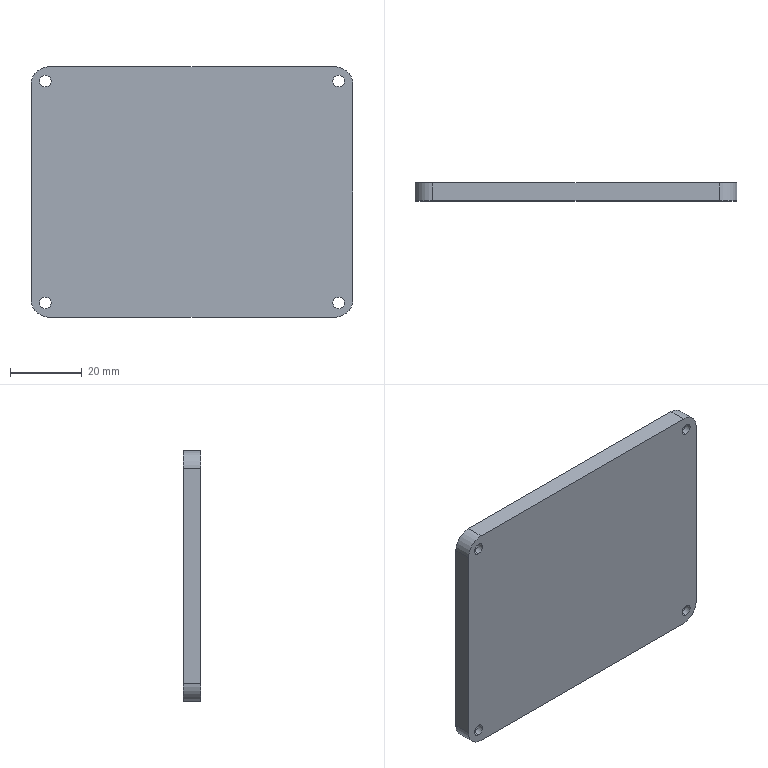Part | SolidWorks | features Extrusion 1, ICE 1 | 1 solid | 30 faces | box 90 x 5 x 70 mm | volume 30997 mm3 | cylinder 20 | plane 10 | commonest cylinder face diameters 3.2 x8 5.8 x8 10 x4
STEP:
#1=CARTESIAN_POINT('',(-41.,1.8,-33.9));
#2=VERTEX_POINT('',#1);
#3=CARTESIAN_POINT('',(-41.,1.8,-28.1));
#4=VERTEX_POINT('',#3);
#5=CARTESIAN_POINT('',(-41.,1.8,-31.));
#6=DIRECTION('',(0.,1.,0.));
#7=DIRECTION('',(0.,0.,1.));
#8=AXIS2_PLACEMENT_3D('',#5,#6,#7);
#9=CIRCLE('',#8,2.9);
#10=EDGE_CURVE('',#2,#4,#9,.T.);
#11=ORIENTED_EDGE('',*,*,#10,.F.);
#12=CARTESIAN_POINT('',(-41.,5.,-33.9));
#13=VERTEX_POINT('',#12);
#14=CARTESIAN_POINT('',(-41.,1.8,-33.9));
#15=DIRECTION('',(0.,1.,0.));
#16=VECTOR('',#15,1000.);
#17=LINE('',#14,#16);
#18=EDGE_CURVE('',#2,#13,#17,.T.);
#19=ORIENTED_EDGE('',*,*,#18,.T.);
#20=CARTESIAN_POINT('',(-41.,5.,-28.1));
#21=VERTEX_POINT('',#20);
#22=CARTESIAN_POINT('',(-41.,5.,-31.));
#23=DIRECTION('',(0.,1.,0.));
#24=DIRECTION('',(0.,0.,1.));
#25=AXIS2_PLACEMENT_3D('',#22,#23,#24);
#26=CIRCLE('',#25,2.9);
#27=EDGE_CURVE('',#13,#21,#26,.T.);
#28=ORIENTED_EDGE('',*,*,#27,.T.);
#29=CARTESIAN_POINT('',(-41.,1.8,-28.1));
#30=DIRECTION('',(0.,1.,0.));
#31=VECTOR('',#30,1000.);
#32=LINE('',#29,#31);
#33=EDGE_CURVE('',#4,#21,#32,.T.);
#34=ORIENTED_EDGE('',*,*,#33,.F.);
#35=EDGE_LOOP('',(#11,#19,#28,#34));
#36=FACE_OUTER_BOUND('',#35,.T.);
#37=CARTESIAN_POINT('',(-41.,1.8,-31.));
#38=DIRECTION('',(0.,1.,0.));
#39=DIRECTION('',(0.,0.,1.));
#40=AXIS2_PLACEMENT_3D('',#37,#38,#39);
#41=CYLINDRICAL_SURFACE('',#40,2.9);
#42=ADVANCED_FACE('',(#36),#41,.F.);
#43=CARTESIAN_POINT('',(-41.,1.8,28.1));
#44=VERTEX_POINT('',#43);
#45=CARTESIAN_POINT('',(-41.,1.8,33.9));
#46=VERTEX_POINT('',#45);
#47=CARTESIAN_POINT('',(-41.,1.8,31.));
#48=DIRECTION('',(0.,1.,0.));
#49=DIRECTION('',(0.,0.,1.));
#50=AXIS2_PLACEMENT_3D('',#47,#48,#49);
#51=CIRCLE('',#50,2.9);
#52=EDGE_CURVE('',#44,#46,#51,.T.);
#53=ORIENTED_EDGE('',*,*,#52,.F.);
#54=CARTESIAN_POINT('',(-41.,5.,28.1));
#55=VERTEX_POINT('',#54);
#56=CARTESIAN_POINT('',(-41.,1.8,28.1));
#57=DIRECTION('',(0.,1.,0.));
#58=VECTOR('',#57,1000.);
#59=LINE('',#56,#58);
#60=EDGE_CURVE('',#44,#55,#59,.T.);
#61=ORIENTED_EDGE('',*,*,#60,.T.);
#62=CARTESIAN_POINT('',(-41.,5.,33.9));
#63=VERTEX_POINT('',#62);
#64=CARTESIAN_POINT('',(-41.,5.,31.));
#65=DIRECTION('',(0.,1.,0.));
#66=DIRECTION('',(0.,0.,1.));
#67=AXIS2_PLACEMENT_3D('',#64,#65,#66);
#68=CIRCLE('',#67,2.9);
#69=EDGE_CURVE('',#55,#63,#68,.T.);
#70=ORIENTED_EDGE('',*,*,#69,.T.);
#71=CARTESIAN_POINT('',(-41.,1.8,33.9));
#72=DIRECTION('',(0.,1.,0.));
#73=VECTOR('',#72,1000.);
#74=LINE('',#71,#73);
#75=EDGE_CURVE('',#46,#63,#74,.T.);
#76=ORIENTED_EDGE('',*,*,#75,.F.);
#77=EDGE_LOOP('',(#53,#61,#70,#76));
#78=FACE_OUTER_BOUND('',#77,.T.);
#79=CARTESIAN_POINT('',(-41.,1.8,31.));
#80=DIRECTION('',(0.,1.,0.));
#81=DIRECTION('',(0.,0.,1.));
#82=AXIS2_PLACEMENT_3D('',#79,#80,#81);
#83=CYLINDRICAL_SURFACE('',#82,2.9);
#84=ADVANCED_FACE('',(#78),#83,.F.);
#85=CARTESIAN_POINT('',(41.,1.8,28.1));
#86=VERTEX_POINT('',#85);
#87=CARTESIAN_POINT('',(41.,1.8,33.9));
#88=VERTEX_POINT('',#87);
#89=CARTESIAN_POINT('',(41.,1.8,31.));
#90=DIRECTION('',(0.,1.,0.));
#91=DIRECTION('',(0.,0.,1.));
#92=AXIS2_PLACEMENT_3D('',#89,#90,#91);
#93=CIRCLE('',#92,2.9);
#94=EDGE_CURVE('',#86,#88,#93,.T.);
#95=ORIENTED_EDGE('',*,*,#94,.F.);
#96=CARTESIAN_POINT('',(41.,5.,28.1));
#97=VERTEX_POINT('',#96);
#98=CARTESIAN_POINT('',(41.,1.8,28.1));
#99=DIRECTION('',(0.,1.,0.));
#100=VECTOR('',#99,1000.);
#101=LINE('',#98,#100);
#102=EDGE_CURVE('',#86,#97,#101,.T.);
#103=ORIENTED_EDGE('',*,*,#102,.T.);
#104=CARTESIAN_POINT('',(41.,5.,33.9));
#105=VERTEX_POINT('',#104);
#106=CARTESIAN_POINT('',(41.,5.,31.));
#107=DIRECTION('',(0.,1.,0.));
#108=DIRECTION('',(0.,0.,1.));
#109=AXIS2_PLACEMENT_3D('',#106,#107,#108);
#110=CIRCLE('',#109,2.9);
#111=EDGE_CURVE('',#97,#105,#110,.T.);
#112=ORIENTED_EDGE('',*,*,#111,.T.);
#113=CARTESIAN_POINT('',(41.,1.8,33.9));
#114=DIRECTION('',(0.,1.,0.));
#115=VECTOR('',#114,1000.);
#116=LINE('',#113,#115);
#117=EDGE_CURVE('',#88,#105,#116,.T.);
#118=ORIENTED_EDGE('',*,*,#117,.F.);
#119=EDGE_LOOP('',(#95,#103,#112,#118));
#120=FACE_OUTER_BOUND('',#119,.T.);
#121=CARTESIAN_POINT('',(41.,1.8,31.));
#122=DIRECTION('',(0.,1.,0.));
#123=DIRECTION('',(0.,0.,1.));
#124=AXIS2_PLACEMENT_3D('',#121,#122,#123);
#125=CYLINDRICAL_SURFACE('',#124,2.9);
#126=ADVANCED_FACE('',(#120),#125,.F.);
#127=CARTESIAN_POINT('',(41.,1.8,-33.9));
#128=VERTEX_POINT('',#127);
#129=CARTESIAN_POINT('',(41.,1.8,-28.1));
#130=VERTEX_POINT('',#129);
#131=CARTESIAN_POINT('',(41.,1.8,-31.));
#132=DIRECTION('',(0.,1.,0.));
#133=DIRECTION('',(0.,0.,1.));
#134=AXIS2_PLACEMENT_3D('',#131,#132,#133);
#135=CIRCLE('',#134,2.9);
#136=EDGE_CURVE('',#128,#130,#135,.T.);
#137=ORIENTED_EDGE('',*,*,#136,.F.);
#138=CARTESIAN_POINT('',(41.,5.,-33.9));
#139=VERTEX_POINT('',#138);
#140=CARTESIAN_POINT('',(41.,1.8,-33.9));
#141=DIRECTION('',(0.,1.,0.));
#142=VECTOR('',#141,1000.);
#143=LINE('',#140,#142);
#144=EDGE_CURVE('',#128,#139,#143,.T.);
#145=ORIENTED_EDGE('',*,*,#144,.T.);
#146=CARTESIAN_POINT('',(41.,5.,-28.1));
#147=VERTEX_POINT('',#146);
#148=CARTESIAN_POINT('',(41.,5.,-31.));
#149=DIRECTION('',(0.,1.,0.));
#150=DIRECTION('',(0.,0.,1.));
#151=AXIS2_PLACEMENT_3D('',#148,#149,#150);
#152=CIRCLE('',#151,2.9);
#153=EDGE_CURVE('',#139,#147,#152,.T.);
#154=ORIENTED_EDGE('',*,*,#153,.T.);
#155=CARTESIAN_POINT('',(41.,1.8,-28.1));
#156=DIRECTION('',(0.,1.,0.));
#157=VECTOR('',#156,1000.);
#158=LINE('',#155,#157);
#159=EDGE_CURVE('',#130,#147,#158,.T.);
#160=ORIENTED_EDGE('',*,*,#159,.F.);
#161=EDGE_LOOP('',(#137,#145,#154,#160));
#162=FACE_OUTER_BOUND('',#161,.T.);
#163=CARTESIAN_POINT('',(41.,1.8,-31.));
#164=DIRECTION('',(0.,1.,0.));
#165=DIRECTION('',(0.,0.,1.));
#166=AXIS2_PLACEMENT_3D('',#163,#164,#165);
#167=CYLINDRICAL_SURFACE('',#166,2.9);
#168=ADVANCED_FACE('',(#162),#167,.F.);
#169=CARTESIAN_POINT('',(41.,1.8,-32.6));
#170=VERTEX_POINT('',#169);
#171=CARTESIAN_POINT('',(41.,1.8,-29.4));
#172=VERTEX_POINT('',#171);
#173=CARTESIAN_POINT('',(41.,1.8,-31.));
#174=DIRECTION('',(0.,1.,0.));
#175=DIRECTION('',(0.,0.,1.));
#176=AXIS2_PLACEMENT_3D('',#173,#174,#175);
#177=CIRCLE('',#176,1.6);
#178=EDGE_CURVE('',#170,#172,#177,.T.);
#179=ORIENTED_EDGE('',*,*,#178,.T.);
#180=CARTESIAN_POINT('',(41.,0.,-29.4));
#181=VERTEX_POINT('',#180);
#182=CARTESIAN_POINT('',(41.,5.,-29.4));
#183=DIRECTION('',(0.,-1.,0.));
#184=VECTOR('',#183,1000.);
#185=LINE('',#182,#184);
#186=EDGE_CURVE('',#172,#181,#185,.T.);
#187=ORIENTED_EDGE('',*,*,#186,.T.);
#188=CARTESIAN_POINT('',(41.,0.,-32.6));
#189=VERTEX_POINT('',#188);
#190=CARTESIAN_POINT('',(41.,0.,-31.));
#191=DIRECTION('',(0.,1.,0.));
#192=DIRECTION('',(0.,0.,1.));
#193=AXIS2_PLACEMENT_3D('',#190,#191,#192);
#194=CIRCLE('',#193,1.6);
#195=EDGE_CURVE('',#189,#181,#194,.T.);
#196=ORIENTED_EDGE('',*,*,#195,.F.);
#197=CARTESIAN_POINT('',(41.,5.,-32.6));
#198=DIRECTION('',(0.,-1.,0.));
#199=VECTOR('',#198,1000.);
#200=LINE('',#197,#199);
#201=EDGE_CURVE('',#170,#189,#200,.T.);
#202=ORIENTED_EDGE('',*,*,#201,.F.);
#203=EDGE_LOOP('',(#179,#187,#196,#202));
#204=FACE_OUTER_BOUND('',#203,.T.);
#205=CARTESIAN_POINT('',(41.,5.,-31.));
#206=DIRECTION('',(0.,-1.,0.));
#207=DIRECTION('',(0.,0.,-1.));
#208=AXIS2_PLACEMENT_3D('',#205,#206,#207);
#209=CYLINDRICAL_SURFACE('',#208,1.6);
#210=ADVANCED_FACE('',(#204),#209,.F.);
#211=CARTESIAN_POINT('',(41.,1.8,29.4));
#212=VERTEX_POINT('',#211);
#213=CARTESIAN_POINT('',(41.,1.8,32.6));
#214=VERTEX_POINT('',#213);
#215=CARTESIAN_POINT('',(41.,1.8,31.));
#216=DIRECTION('',(0.,1.,0.));
#217=DIRECTION('',(0.,0.,1.));
#218=AXIS2_PLACEMENT_3D('',#215,#216,#217);
#219=CIRCLE('',#218,1.6);
#220=EDGE_CURVE('',#212,#214,#219,.T.);
#221=ORIENTED_EDGE('',*,*,#220,.T.);
#222=CARTESIAN_POINT('',(41.,0.,32.6));
#223=VERTEX_POINT('',#222);
#224=CARTESIAN_POINT('',(41.,5.,32.6));
#225=DIRECTION('',(0.,-1.,0.));
#226=VECTOR('',#225,1000.);
#227=LINE('',#224,#226);
#228=EDGE_CURVE('',#214,#223,#227,.T.);
#229=ORIENTED_EDGE('',*,*,#228,.T.);
#230=CARTESIAN_POINT('',(41.,0.,29.4));
#231=VERTEX_POINT('',#230);
#232=CARTESIAN_POINT('',(41.,0.,31.));
#233=DIRECTION('',(0.,1.,0.));
#234=DIRECTION('',(0.,0.,1.));
#235=AXIS2_PLACEMENT_3D('',#232,#233,#234);
#236=CIRCLE('',#235,1.6);
#237=EDGE_CURVE('',#231,#223,#236,.T.);
#238=ORIENTED_EDGE('',*,*,#237,.F.);
#239=CARTESIAN_POINT('',(41.,5.,29.4));
#240=DIRECTION('',(0.,-1.,0.));
#241=VECTOR('',#240,1000.);
#242=LINE('',#239,#241);
#243=EDGE_CURVE('',#212,#231,#242,.T.);
#244=ORIENTED_EDGE('',*,*,#243,.F.);
#245=EDGE_LOOP('',(#221,#229,#238,#244));
#246=FACE_OUTER_BOUND('',#245,.T.);
#247=CARTESIAN_POINT('',(41.,5.,31.));
#248=DIRECTION('',(0.,-1.,0.));
#249=DIRECTION('',(0.,0.,-1.));
#250=AXIS2_PLACEMENT_3D('',#247,#248,#249);
#251=CYLINDRICAL_SURFACE('',#250,1.6);
#252=ADVANCED_FACE('',(#246),#251,.F.);
#253=CARTESIAN_POINT('',(-41.,1.8,29.4));
#254=VERTEX_POINT('',#253);
#255=CARTESIAN_POINT('',(-41.,1.8,32.6));
#256=VERTEX_POINT('',#255);
#257=CARTESIAN_POINT('',(-41.,1.8,31.));
#258=DIRECTION('',(0.,1.,0.));
#259=DIRECTION('',(0.,0.,1.));
#260=AXIS2_PLACEMENT_3D('',#257,#258,#259);
#261=CIRCLE('',#260,1.6);
#262=EDGE_CURVE('',#254,#256,#261,.T.);
#263=ORIENTED_EDGE('',*,*,#262,.T.);
#264=CARTESIAN_POINT('',(-41.,0.,32.6));
#265=VERTEX_POINT('',#264);
#266=CARTESIAN_POINT('',(-41.,5.,32.6));
#267=DIRECTION('',(0.,-1.,0.));
#268=VECTOR('',#267,1000.);
#269=LINE('',#266,#268);
#270=EDGE_CURVE('',#256,#265,#269,.T.);
#271=ORIENTED_EDGE('',*,*,#270,.T.);
#272=CARTESIAN_POINT('',(-41.,0.,29.4));
#273=VERTEX_POINT('',#272);
#274=CARTESIAN_POINT('',(-41.,0.,31.));
#275=DIRECTION('',(0.,1.,0.));
#276=DIRECTION('',(0.,0.,1.));
#277=AXIS2_PLACEMENT_3D('',#274,#275,#276);
#278=CIRCLE('',#277,1.6);
#279=EDGE_CURVE('',#273,#265,#278,.T.);
#280=ORIENTED_EDGE('',*,*,#279,.F.);
#281=CARTESIAN_POINT('',(-41.,5.,29.4));
#282=DIRECTION('',(0.,-1.,0.));
#283=VECTOR('',#282,1000.);
#284=LINE('',#281,#283);
#285=EDGE_CURVE('',#254,#273,#284,.T.);
#286=ORIENTED_EDGE('',*,*,#285,.F.);
#287=EDGE_LOOP('',(#263,#271,#280,#286));
#288=FACE_OUTER_BOUND('',#287,.T.);
#289=CARTESIAN_POINT('',(-41.,5.,31.));
#290=DIRECTION('',(0.,-1.,0.));
#291=DIRECTION('',(0.,0.,-1.));
#292=AXIS2_PLACEMENT_3D('',#289,#290,#291);
#293=CYLINDRICAL_SURFACE('',#292,1.6);
#294=ADVANCED_FACE('',(#288),#293,.F.);
#295=CARTESIAN_POINT('',(-41.,1.8,-32.6));
#296=VERTEX_POINT('',#295);
#297=CARTESIAN_POINT('',(-41.,1.8,-29.4));
#298=VERTEX_POINT('',#297);
#299=CARTESIAN_POINT('',(-41.,1.8,-31.));
#300=DIRECTION('',(0.,1.,0.));
#301=DIRECTION('',(0.,0.,1.));
#302=AXIS2_PLACEMENT_3D('',#299,#300,#301);
#303=CIRCLE('',#302,1.6);
#304=EDGE_CURVE('',#296,#298,#303,.T.);
#305=ORIENTED_EDGE('',*,*,#304,.T.);
#306=CARTESIAN_POINT('',(-41.,0.,-29.4));
#307=VERTEX_POINT('',#306);
#308=CARTESIAN_POINT('',(-41.,5.,-29.4));
#309=DIRECTION('',(0.,-1.,0.));
#310=VECTOR('',#309,1000.);
#311=LINE('',#308,#310);
#312=EDGE_CURVE('',#298,#307,#311,.T.);
#313=ORIENTED_EDGE('',*,*,#312,.T.);
#314=CARTESIAN_POINT('',(-41.,0.,-32.6));
#315=VERTEX_POINT('',#314);
#316=CARTESIAN_POINT('',(-41.,0.,-31.));
#317=DIRECTION('',(0.,1.,0.));
#318=DIRECTION('',(0.,0.,1.));
#319=AXIS2_PLACEMENT_3D('',#316,#317,#318);
#320=CIRCLE('',#319,1.6);
#321=EDGE_CURVE('',#315,#307,#320,.T.);
#322=ORIENTED_EDGE('',*,*,#321,.F.);
#323=CARTESIAN_POINT('',(-41.,5.,-32.6));
#324=DIRECTION('',(0.,-1.,0.));
#325=VECTOR('',#324,1000.);
#326=LINE('',#323,#325);
#327=EDGE_CURVE('',#296,#315,#326,.T.);
#328=ORIENTED_EDGE('',*,*,#327,.F.);
#329=EDGE_LOOP('',(#305,#313,#322,#328));
#330=FACE_OUTER_BOUND('',#329,.T.);
#331=CARTESIAN_POINT('',(-41.,5.,-31.));
#332=DIRECTION('',(0.,-1.,0.));
#333=DIRECTION('',(0.,0.,-1.));
#334=AXIS2_PLACEMENT_3D('',#331,#332,#333);
#335=CYLINDRICAL_SURFACE('',#334,1.6);
#336=ADVANCED_FACE('',(#330),#335,.F.);
#337=ORIENTED_EDGE('',*,*,#312,.F.);
#338=CARTESIAN_POINT('',(-41.,1.8,-31.));
#339=DIRECTION('',(0.,1.,0.));
#340=DIRECTION('',(0.,0.,1.));
#341=AXIS2_PLACEMENT_3D('',#338,#339,#340);
#342=CIRCLE('',#341,1.6);
#343=EDGE_CURVE('',#298,#296,#342,.T.);
#344=ORIENTED_EDGE('',*,*,#343,.T.);
#345=ORIENTED_EDGE('',*,*,#327,.T.);
#346=CARTESIAN_POINT('',(-41.,0.,-31.));
#347=DIRECTION('',(0.,1.,0.));
#348=DIRECTION('',(0.,0.,1.));
#349=AXIS2_PLACEMENT_3D('',#346,#347,#348);
#350=CIRCLE('',#349,1.6);
#351=EDGE_CURVE('',#307,#315,#350,.T.);
#352=ORIENTED_EDGE('',*,*,#351,.F.);
#353=EDGE_LOOP('',(#337,#344,#345,#352));
#354=FACE_OUTER_BOUND('',#353,.T.);
#355=CARTESIAN_POINT('',(-41.,5.,-31.));
#356=DIRECTION('',(0.,-1.,0.));
#357=DIRECTION('',(0.,0.,-1.));
#358=AXIS2_PLACEMENT_3D('',#355,#356,#357);
#359=CYLINDRICAL_SURFACE('',#358,1.6);
#360=ADVANCED_FACE('',(#354),#359,.F.);
#361=ORIENTED_EDGE('',*,*,#270,.F.);
#362=CARTESIAN_POINT('',(-41.,1.8,31.));
#363=DIRECTION('',(0.,1.,0.));
#364=DIRECTION('',(0.,0.,1.));
#365=AXIS2_PLACEMENT_3D('',#362,#363,#364);
#366=CIRCLE('',#365,1.6);
#367=EDGE_CURVE('',#256,#254,#366,.T.);
#368=ORIENTED_EDGE('',*,*,#367,.T.);
#369=ORIENTED_EDGE('',*,*,#285,.T.);
#370=CARTESIAN_POINT('',(-41.,0.,31.));
#371=DIRECTION('',(0.,1.,0.));
#372=DIRECTION('',(0.,0.,1.));
#373=AXIS2_PLACEMENT_3D('',#370,#371,#372);
#374=CIRCLE('',#373,1.6);
#375=EDGE_CURVE('',#265,#273,#374,.T.);
#376=ORIENTED_EDGE('',*,*,#375,.F.);
#377=EDGE_LOOP('',(#361,#368,#369,#376));
#378=FACE_OUTER_BOUND('',#377,.T.);
#379=CARTESIAN_POINT('',(-41.,5.,31.));
#380=DIRECTION('',(0.,-1.,0.));
#381=DIRECTION('',(0.,0.,-1.));
#382=AXIS2_PLACEMENT_3D('',#379,#380,#381);
#383=CYLINDRICAL_SURFACE('',#382,1.6);
#384=ADVANCED_FACE('',(#378),#383,.F.);
#385=ORIENTED_EDGE('',*,*,#228,.F.);
#386=CARTESIAN_POINT('',(41.,1.8,31.));
#387=DIRECTION('',(0.,1.,0.));
#388=DIRECTION('',(0.,0.,1.));
#389=AXIS2_PLACEMENT_3D('',#386,#387,#388);
#390=CIRCLE('',#389,1.6);
#391=EDGE_CURVE('',#214,#212,#390,.T.);
#392=ORIENTED_EDGE('',*,*,#391,.T.);
#393=ORIENTED_EDGE('',*,*,#243,.T.);
#394=CARTESIAN_POINT('',(41.,0.,31.));
#395=DIRECTION('',(0.,1.,0.));
#396=DIRECTION('',(0.,0.,1.));
#397=AXIS2_PLACEMENT_3D('',#394,#395,#396);
#398=CIRCLE('',#397,1.6);
#399=EDGE_CURVE('',#223,#231,#398,.T.);
#400=ORIENTED_EDGE('',*,*,#399,.F.);
#401=EDGE_LOOP('',(#385,#392,#393,#400));
#402=FACE_OUTER_BOUND('',#401,.T.);
#403=CARTESIAN_POINT('',(41.,5.,31.));
#404=DIRECTION('',(0.,-1.,0.));
#405=DIRECTION('',(0.,0.,-1.));
#406=AXIS2_PLACEMENT_3D('',#403,#404,#405);
#407=CYLINDRICAL_SURFACE('',#406,1.6);
#408=ADVANCED_FACE('',(#402),#407,.F.);
#409=ORIENTED_EDGE('',*,*,#186,.F.);
#410=CARTESIAN_POINT('',(41.,1.8,-31.));
#411=DIRECTION('',(0.,1.,0.));
#412=DIRECTION('',(0.,0.,1.));
#413=AXIS2_PLACEMENT_3D('',#410,#411,#412);
#414=CIRCLE('',#413,1.6);
#415=EDGE_CURVE('',#172,#170,#414,.T.);
#416=ORIENTED_EDGE('',*,*,#415,.T.);
#417=ORIENTED_EDGE('',*,*,#201,.T.);
#418=CARTESIAN_POINT('',(41.,0.,-31.));
#419=DIRECTION('',(0.,1.,0.));
#420=DIRECTION('',(0.,0.,1.));
#421=AXIS2_PLACEMENT_3D('',#418,#419,#420);
#422=CIRCLE('',#421,1.6);
#423=EDGE_CURVE('',#181,#189,#422,.T.);
#424=ORIENTED_EDGE('',*,*,#423,.F.);
#425=EDGE_LOOP('',(#409,#416,#417,#424));
#426=FACE_OUTER_BOUND('',#425,.T.);
#427=CARTESIAN_POINT('',(41.,5.,-31.));
#428=DIRECTION('',(0.,-1.,0.));
#429=DIRECTION('',(0.,0.,-1.));
#430=AXIS2_PLACEMENT_3D('',#427,#428,#429);
#431=CYLINDRICAL_SURFACE('',#430,1.6);
#432=ADVANCED_FACE('',(#426),#431,.F.);
#433=CARTESIAN_POINT('',(41.,5.,31.));
#434=DIRECTION('',(0.,1.,0.));
#435=DIRECTION('',(0.,0.,1.));
#436=AXIS2_PLACEMENT_3D('',#433,#434,#435);
#437=CIRCLE('',#436,2.9);
#438=EDGE_CURVE('',#105,#97,#437,.T.);
#439=ORIENTED_EDGE('',*,*,#438,.F.);
#440=ORIENTED_EDGE('',*,*,#111,.F.);
#441=EDGE_LOOP('',(#439,#440));
#442=FACE_BOUND('',#441,.T.);
#443=CARTESIAN_POINT('',(-41.,5.,31.));
#444=DIRECTION('',(0.,1.,0.));
#445=DIRECTION('',(0.,0.,1.));
#446=AXIS2_PLACEMENT_3D('',#443,#444,#445);
#447=CIRCLE('',#446,2.9);
#448=EDGE_CURVE('',#63,#55,#447,.T.);
#449=ORIENTED_EDGE('',*,*,#448,.F.);
#450=ORIENTED_EDGE('',*,*,#69,.F.);
#451=EDGE_LOOP('',(#449,#450));
#452=FACE_BOUND('',#451,.T.);
#453=CARTESIAN_POINT('',(-41.,5.,-31.));
#454=DIRECTION('',(0.,1.,0.));
#455=DIRECTION('',(0.,0.,1.));
#456=AXIS2_PLACEMENT_3D('',#453,#454,#455);
#457=CIRCLE('',#456,2.9);
#458=EDGE_CURVE('',#21,#13,#457,.T.);
#459=ORIENTED_EDGE('',*,*,#458,.F.);
#460=ORIENTED_EDGE('',*,*,#27,.F.);
#461=EDGE_LOOP('',(#459,#460));
#462=FACE_BOUND('',#461,.T.);
#463=CARTESIAN_POINT('',(41.,5.,-31.));
#464=DIRECTION('',(0.,1.,0.));
#465=DIRECTION('',(0.,0.,1.));
#466=AXIS2_PLACEMENT_3D('',#463,#464,#465);
#467=CIRCLE('',#466,2.9);
#468=EDGE_CURVE('',#147,#139,#467,.T.);
#469=ORIENTED_EDGE('',*,*,#468,.F.);
#470=ORIENTED_EDGE('',*,*,#153,.F.);
#471=EDGE_LOOP('',(#469,#470));
#472=FACE_BOUND('',#471,.T.);
#473=CARTESIAN_POINT('',(-45.,5.,30.));
#474=VERTEX_POINT('',#473);
#475=CARTESIAN_POINT('',(-40.,5.,35.));
#476=VERTEX_POINT('',#475);
#477=CARTESIAN_POINT('',(-40.,5.,30.));
#478=DIRECTION('',(0.,1.,0.));
#479=DIRECTION('',(0.,0.,-1.));
#480=AXIS2_PLACEMENT_3D('',#477,#478,#479);
#481=CIRCLE('',#480,5.);
#482=EDGE_CURVE('',#474,#476,#481,.T.);
#483=ORIENTED_EDGE('',*,*,#482,.T.);
#484=CARTESIAN_POINT('',(40.,5.,35.));
#485=VERTEX_POINT('',#484);
#486=CARTESIAN_POINT('',(-40.,5.,35.));
#487=DIRECTION('',(1.,0.,0.));
#488=VECTOR('',#487,1000.);
#489=LINE('',#486,#488);
#490=EDGE_CURVE('',#476,#485,#489,.T.);
#491=ORIENTED_EDGE('',*,*,#490,.T.);
#492=CARTESIAN_POINT('',(45.,5.,30.));
#493=VERTEX_POINT('',#492);
#494=CARTESIAN_POINT('',(40.,5.,30.));
#495=DIRECTION('',(0.,1.,0.));
#496=DIRECTION('',(0.,0.,1.));
#497=AXIS2_PLACEMENT_3D('',#494,#495,#496);
#498=CIRCLE('',#497,5.);
#499=EDGE_CURVE('',#485,#493,#498,.T.);
#500=ORIENTED_EDGE('',*,*,#499,.T.);
#501=CARTESIAN_POINT('',(45.,5.,-30.));
#502=VERTEX_POINT('',#501);
#503=CARTESIAN_POINT('',(45.,5.,30.));
#504=DIRECTION('',(0.,0.,-1.));
#505=VECTOR('',#504,1000.);
#506=LINE('',#503,#505);
#507=EDGE_CURVE('',#493,#502,#506,.T.);
#508=ORIENTED_EDGE('',*,*,#507,.T.);
#509=CARTESIAN_POINT('',(40.,5.,-35.));
#510=VERTEX_POINT('',#509);
#511=CARTESIAN_POINT('',(40.,5.,-30.));
#512=DIRECTION('',(0.,1.,0.));
#513=DIRECTION('',(0.,0.,-1.));
#514=AXIS2_PLACEMENT_3D('',#511,#512,#513);
#515=CIRCLE('',#514,5.);
#516=EDGE_CURVE('',#502,#510,#515,.T.);
#517=ORIENTED_EDGE('',*,*,#516,.T.);
#518=CARTESIAN_POINT('',(-40.,5.,-35.));
#519=VERTEX_POINT('',#518);
#520=CARTESIAN_POINT('',(-40.,5.,-35.));
#521=DIRECTION('',(-1.,0.,0.));
#522=VECTOR('',#521,1000.);
#523=LINE('',#520,#522);
#524=EDGE_CURVE('',#510,#519,#523,.T.);
#525=ORIENTED_EDGE('',*,*,#524,.T.);
#526=CARTESIAN_POINT('',(-45.,5.,-30.));
#527=VERTEX_POINT('',#526);
#528=CARTESIAN_POINT('',(-40.,5.,-30.));
#529=DIRECTION('',(0.,1.,0.));
#530=DIRECTION('',(0.,0.,-1.));
#531=AXIS2_PLACEMENT_3D('',#528,#529,#530);
#532=CIRCLE('',#531,5.);
#533=EDGE_CURVE('',#519,#527,#532,.T.);
#534=ORIENTED_EDGE('',*,*,#533,.T.);
#535=CARTESIAN_POINT('',(-45.,5.,30.));
#536=DIRECTION('',(0.,0.,1.));
#537=VECTOR('',#536,1000.);
#538=LINE('',#535,#537);
#539=EDGE_CURVE('',#527,#474,#538,.T.);
#540=ORIENTED_EDGE('',*,*,#539,.T.);
#541=EDGE_LOOP('',(#483,#491,#500,#508,#517,#525,#534,#540));
#542=FACE_OUTER_BOUND('',#541,.T.);
#543=CARTESIAN_POINT('',(-40.,5.,30.));
#544=DIRECTION('',(0.,-1.,0.));
#545=DIRECTION('',(0.,0.,-1.));
#546=AXIS2_PLACEMENT_3D('',#543,#544,#545);
#547=PLANE('',#546);
#548=ADVANCED_FACE('',(#442,#452,#462,#472,#542),#547,.F.);
#549=ORIENTED_EDGE('',*,*,#237,.T.);
#550=ORIENTED_EDGE('',*,*,#399,.T.);
#551=EDGE_LOOP('',(#549,#550));
#552=FACE_BOUND('',#551,.T.);
#553=ORIENTED_EDGE('',*,*,#321,.T.);
#554=ORIENTED_EDGE('',*,*,#351,.T.);
#555=EDGE_LOOP('',(#553,#554));
#556=FACE_BOUND('',#555,.T.);
#557=CARTESIAN_POINT('',(-45.,0.,30.));
#558=VERTEX_POINT('',#557);
#559=CARTESIAN_POINT('',(-40.,0.,35.));
#560=VERTEX_POINT('',#559);
#561=CARTESIAN_POINT('',(-40.,0.,30.));
#562=DIRECTION('',(0.,1.,0.));
#563=DIRECTION('',(0.,0.,-1.));
#564=AXIS2_PLACEMENT_3D('',#561,#562,#563);
#565=CIRCLE('',#564,5.);
#566=EDGE_CURVE('',#558,#560,#565,.T.);
#567=ORIENTED_EDGE('',*,*,#566,.F.);
#568=CARTESIAN_POINT('',(-45.,0.,-30.));
#569=VERTEX_POINT('',#568);
#570=CARTESIAN_POINT('',(-45.,0.,30.));
#571=DIRECTION('',(0.,0.,1.));
#572=VECTOR('',#571,1000.);
#573=LINE('',#570,#572);
#574=EDGE_CURVE('',#569,#558,#573,.T.);
#575=ORIENTED_EDGE('',*,*,#574,.F.);
#576=CARTESIAN_POINT('',(-40.,0.,-35.));
#577=VERTEX_POINT('',#576);
#578=CARTESIAN_POINT('',(-40.,0.,-30.));
#579=DIRECTION('',(0.,1.,0.));
#580=DIRECTION('',(0.,0.,-1.));
#581=AXIS2_PLACEMENT_3D('',#578,#579,#580);
#582=CIRCLE('',#581,5.);
#583=EDGE_CURVE('',#577,#569,#582,.T.);
#584=ORIENTED_EDGE('',*,*,#583,.F.);
#585=CARTESIAN_POINT('',(40.,0.,-35.));
#586=VERTEX_POINT('',#585);
#587=CARTESIAN_POINT('',(-40.,0.,-35.));
#588=DIRECTION('',(-1.,0.,0.));
#589=VECTOR('',#588,1000.);
#590=LINE('',#587,#589);
#591=EDGE_CURVE('',#586,#577,#590,.T.);
#592=ORIENTED_EDGE('',*,*,#591,.F.);
#593=CARTESIAN_POINT('',(45.,0.,-30.));
#594=VERTEX_POINT('',#593);
#595=CARTESIAN_POINT('',(40.,0.,-30.));
#596=DIRECTION('',(0.,1.,0.));
#597=DIRECTION('',(0.,0.,-1.));
#598=AXIS2_PLACEMENT_3D('',#595,#596,#597);
#599=CIRCLE('',#598,5.);
#600=EDGE_CURVE('',#594,#586,#599,.T.);
#601=ORIENTED_EDGE('',*,*,#600,.F.);
#602=CARTESIAN_POINT('',(45.,0.,30.));
#603=VERTEX_POINT('',#602);
#604=CARTESIAN_POINT('',(45.,0.,30.));
#605=DIRECTION('',(0.,0.,-1.));
#606=VECTOR('',#605,1000.);
#607=LINE('',#604,#606);
#608=EDGE_CURVE('',#603,#594,#607,.T.);
#609=ORIENTED_EDGE('',*,*,#608,.F.);
#610=CARTESIAN_POINT('',(40.,0.,35.));
#611=VERTEX_POINT('',#610);
#612=CARTESIAN_POINT('',(40.,0.,30.));
#613=DIRECTION('',(0.,1.,0.));
#614=DIRECTION('',(0.,0.,1.));
#615=AXIS2_PLACEMENT_3D('',#612,#613,#614);
#616=CIRCLE('',#615,5.);
#617=EDGE_CURVE('',#611,#603,#616,.T.);
#618=ORIENTED_EDGE('',*,*,#617,.F.);
#619=CARTESIAN_POINT('',(-40.,0.,35.));
#620=DIRECTION('',(1.,0.,0.));
#621=VECTOR('',#620,1000.);
#622=LINE('',#619,#621);
#623=EDGE_CURVE('',#560,#611,#622,.T.);
#624=ORIENTED_EDGE('',*,*,#623,.F.);
#625=EDGE_LOOP('',(#567,#575,#584,#592,#601,#609,#618,#624));
#626=FACE_OUTER_BOUND('',#625,.T.);
#627=ORIENTED_EDGE('',*,*,#279,.T.);
#628=ORIENTED_EDGE('',*,*,#375,.T.);
#629=EDGE_LOOP('',(#627,#628));
#630=FACE_BOUND('',#629,.T.);
#631=ORIENTED_EDGE('',*,*,#195,.T.);
#632=ORIENTED_EDGE('',*,*,#423,.T.);
#633=EDGE_LOOP('',(#631,#632));
#634=FACE_BOUND('',#633,.T.);
#635=CARTESIAN_POINT('',(-40.,0.,30.));
#636=DIRECTION('',(0.,-1.,0.));
#637=DIRECTION('',(0.,0.,-1.));
#638=AXIS2_PLACEMENT_3D('',#635,#636,#637);
#639=PLANE('',#638);
#640=ADVANCED_FACE('',(#552,#556,#626,#630,#634),#639,.T.);
#641=ORIENTED_EDGE('',*,*,#566,.T.);
#642=CARTESIAN_POINT('',(-40.,5.,35.));
#643=DIRECTION('',(0.,-1.,0.));
#644=VECTOR('',#643,1000.);
#645=LINE('',#642,#644);
#646=EDGE_CURVE('',#476,#560,#645,.T.);
#647=ORIENTED_EDGE('',*,*,#646,.F.);
#648=ORIENTED_EDGE('',*,*,#482,.F.);
#649=CARTESIAN_POINT('',(-45.,5.,30.));
#650=DIRECTION('',(0.,-1.,0.));
#651=VECTOR('',#650,1000.);
#652=LINE('',#649,#651);
#653=EDGE_CURVE('',#474,#558,#652,.T.);
#654=ORIENTED_EDGE('',*,*,#653,.T.);
#655=EDGE_LOOP('',(#641,#647,#648,#654));
#656=FACE_OUTER_BOUND('',#655,.T.);
#657=CARTESIAN_POINT('',(-40.,5.,30.));
#658=DIRECTION('',(0.,-1.,0.));
#659=DIRECTION('',(0.,0.,-1.));
#660=AXIS2_PLACEMENT_3D('',#657,#658,#659);
#661=CYLINDRICAL_SURFACE('',#660,5.);
#662=ADVANCED_FACE('',(#656),#661,.T.);
#663=ORIENTED_EDGE('',*,*,#623,.T.);
#664=CARTESIAN_POINT('',(40.,5.,35.));
#665=DIRECTION('',(0.,-1.,0.));
#666=VECTOR('',#665,1000.);
#667=LINE('',#664,#666);
#668=EDGE_CURVE('',#485,#611,#667,.T.);
#669=ORIENTED_EDGE('',*,*,#668,.F.);
#670=ORIENTED_EDGE('',*,*,#490,.F.);
#671=ORIENTED_EDGE('',*,*,#646,.T.);
#672=EDGE_LOOP('',(#663,#669,#670,#671));
#673=FACE_OUTER_BOUND('',#672,.T.);
#674=CARTESIAN_POINT('',(-40.,5.,35.));
#675=DIRECTION('',(0.,0.,-1.));
#676=DIRECTION('',(-1.,0.,0.));
#677=AXIS2_PLACEMENT_3D('',#674,#675,#676);
#678=PLANE('',#677);
#679=ADVANCED_FACE('',(#673),#678,.F.);
#680=ORIENTED_EDGE('',*,*,#617,.T.);
#681=CARTESIAN_POINT('',(45.,5.,30.));
#682=DIRECTION('',(0.,-1.,0.));
#683=VECTOR('',#682,1000.);
#684=LINE('',#681,#683);
#685=EDGE_CURVE('',#493,#603,#684,.T.);
#686=ORIENTED_EDGE('',*,*,#685,.F.);
#687=ORIENTED_EDGE('',*,*,#499,.F.);
#688=ORIENTED_EDGE('',*,*,#668,.T.);
#689=EDGE_LOOP('',(#680,#686,#687,#688));
#690=FACE_OUTER_BOUND('',#689,.T.);
#691=CARTESIAN_POINT('',(40.,5.,30.));
#692=DIRECTION('',(0.,-1.,0.));
#693=DIRECTION('',(0.,0.,-1.));
#694=AXIS2_PLACEMENT_3D('',#691,#692,#693);
#695=CYLINDRICAL_SURFACE('',#694,5.);
#696=ADVANCED_FACE('',(#690),#695,.T.);
#697=ORIENTED_EDGE('',*,*,#608,.T.);
#698=CARTESIAN_POINT('',(45.,5.,-30.));
#699=DIRECTION('',(0.,-1.,0.));
#700=VECTOR('',#699,1000.);
#701=LINE('',#698,#700);
#702=EDGE_CURVE('',#502,#594,#701,.T.);
#703=ORIENTED_EDGE('',*,*,#702,.F.);
#704=ORIENTED_EDGE('',*,*,#507,.F.);
#705=ORIENTED_EDGE('',*,*,#685,.T.);
#706=EDGE_LOOP('',(#697,#703,#704,#705));
#707=FACE_OUTER_BOUND('',#706,.T.);
#708=CARTESIAN_POINT('',(45.,5.,30.));
#709=DIRECTION('',(-1.,0.,0.));
#710=DIRECTION('',(0.,0.,1.));
#711=AXIS2_PLACEMENT_3D('',#708,#709,#710);
#712=PLANE('',#711);
#713=ADVANCED_FACE('',(#707),#712,.F.);
#714=ORIENTED_EDGE('',*,*,#600,.T.);
#715=CARTESIAN_POINT('',(40.,5.,-35.));
#716=DIRECTION('',(0.,-1.,0.));
#717=VECTOR('',#716,1000.);
#718=LINE('',#715,#717);
#719=EDGE_CURVE('',#510,#586,#718,.T.);
#720=ORIENTED_EDGE('',*,*,#719,.F.);
#721=ORIENTED_EDGE('',*,*,#516,.F.);
#722=ORIENTED_EDGE('',*,*,#702,.T.);
#723=EDGE_LOOP('',(#714,#720,#721,#722));
#724=FACE_OUTER_BOUND('',#723,.T.);
#725=CARTESIAN_POINT('',(40.,5.,-30.));
#726=DIRECTION('',(0.,-1.,0.));
#727=DIRECTION('',(0.,0.,-1.));
#728=AXIS2_PLACEMENT_3D('',#725,#726,#727);
#729=CYLINDRICAL_SURFACE('',#728,5.);
#730=ADVANCED_FACE('',(#724),#729,.T.);
#731=ORIENTED_EDGE('',*,*,#591,.T.);
#732=CARTESIAN_POINT('',(-40.,5.,-35.));
#733=DIRECTION('',(0.,-1.,0.));
#734=VECTOR('',#733,1000.);
#735=LINE('',#732,#734);
#736=EDGE_CURVE('',#519,#577,#735,.T.);
#737=ORIENTED_EDGE('',*,*,#736,.F.);
#738=ORIENTED_EDGE('',*,*,#524,.F.);
#739=ORIENTED_EDGE('',*,*,#719,.T.);
#740=EDGE_LOOP('',(#731,#737,#738,#739));
#741=FACE_OUTER_BOUND('',#740,.T.);
#742=CARTESIAN_POINT('',(-40.,5.,-35.));
#743=DIRECTION('',(0.,0.,1.));
#744=DIRECTION('',(1.,0.,0.));
#745=AXIS2_PLACEMENT_3D('',#742,#743,#744);
#746=PLANE('',#745);
#747=ADVANCED_FACE('',(#741),#746,.F.);
#748=ORIENTED_EDGE('',*,*,#583,.T.);
#749=CARTESIAN_POINT('',(-45.,5.,-30.));
#750=DIRECTION('',(0.,-1.,0.));
#751=VECTOR('',#750,1000.);
#752=LINE('',#749,#751);
#753=EDGE_CURVE('',#527,#569,#752,.T.);
#754=ORIENTED_EDGE('',*,*,#753,.F.);
#755=ORIENTED_EDGE('',*,*,#533,.F.);
#756=ORIENTED_EDGE('',*,*,#736,.T.);
#757=EDGE_LOOP('',(#748,#754,#755,#756));
#758=FACE_OUTER_BOUND('',#757,.T.);
#759=CARTESIAN_POINT('',(-40.,5.,-30.));
#760=DIRECTION('',(0.,-1.,0.));
#761=DIRECTION('',(0.,0.,-1.));
#762=AXIS2_PLACEMENT_3D('',#759,#760,#761);
#763=CYLINDRICAL_SURFACE('',#762,5.);
#764=ADVANCED_FACE('',(#758),#763,.T.);
#765=ORIENTED_EDGE('',*,*,#574,.T.);
#766=ORIENTED_EDGE('',*,*,#653,.F.);
#767=ORIENTED_EDGE('',*,*,#539,.F.);
#768=ORIENTED_EDGE('',*,*,#753,.T.);
#769=EDGE_LOOP('',(#765,#766,#767,#768));
#770=FACE_OUTER_BOUND('',#769,.T.);
#771=CARTESIAN_POINT('',(-45.,5.,30.));
#772=DIRECTION('',(1.,0.,0.));
#773=DIRECTION('',(0.,0.,-1.));
#774=AXIS2_PLACEMENT_3D('',#771,#772,#773);
#775=PLANE('',#774);
#776=ADVANCED_FACE('',(#770),#775,.F.);
#777=ORIENTED_EDGE('',*,*,#144,.F.);
#778=CARTESIAN_POINT('',(41.,1.8,-31.));
#779=DIRECTION('',(0.,1.,0.));
#780=DIRECTION('',(0.,0.,1.));
#781=AXIS2_PLACEMENT_3D('',#778,#779,#780);
#782=CIRCLE('',#781,2.9);
#783=EDGE_CURVE('',#130,#128,#782,.T.);
#784=ORIENTED_EDGE('',*,*,#783,.F.);
#785=ORIENTED_EDGE('',*,*,#159,.T.);
#786=ORIENTED_EDGE('',*,*,#468,.T.);
#787=EDGE_LOOP('',(#777,#784,#785,#786));
#788=FACE_OUTER_BOUND('',#787,.T.);
#789=CARTESIAN_POINT('',(41.,1.8,-31.));
#790=DIRECTION('',(0.,1.,0.));
#791=DIRECTION('',(0.,0.,1.));
#792=AXIS2_PLACEMENT_3D('',#789,#790,#791);
#793=CYLINDRICAL_SURFACE('',#792,2.9);
#794=ADVANCED_FACE('',(#788),#793,.F.);
#795=ORIENTED_EDGE('',*,*,#178,.F.);
#796=ORIENTED_EDGE('',*,*,#415,.F.);
#797=EDGE_LOOP('',(#795,#796));
#798=FACE_BOUND('',#797,.T.);
#799=ORIENTED_EDGE('',*,*,#783,.T.);
#800=ORIENTED_EDGE('',*,*,#136,.T.);
#801=EDGE_LOOP('',(#799,#800));
#802=FACE_OUTER_BOUND('',#801,.T.);
#803=CARTESIAN_POINT('',(41.,1.8,-31.));
#804=DIRECTION('',(0.,1.,0.));
#805=DIRECTION('',(0.,0.,1.));
#806=AXIS2_PLACEMENT_3D('',#803,#804,#805);
#807=PLANE('',#806);
#808=ADVANCED_FACE('',(#798,#802),#807,.T.);
#809=ORIENTED_EDGE('',*,*,#102,.F.);
#810=CARTESIAN_POINT('',(41.,1.8,31.));
#811=DIRECTION('',(0.,1.,0.));
#812=DIRECTION('',(0.,0.,1.));
#813=AXIS2_PLACEMENT_3D('',#810,#811,#812);
#814=CIRCLE('',#813,2.9);
#815=EDGE_CURVE('',#88,#86,#814,.T.);
#816=ORIENTED_EDGE('',*,*,#815,.F.);
#817=ORIENTED_EDGE('',*,*,#117,.T.);
#818=ORIENTED_EDGE('',*,*,#438,.T.);
#819=EDGE_LOOP('',(#809,#816,#817,#818));
#820=FACE_OUTER_BOUND('',#819,.T.);
#821=CARTESIAN_POINT('',(41.,1.8,31.));
#822=DIRECTION('',(0.,1.,0.));
#823=DIRECTION('',(0.,0.,1.));
#824=AXIS2_PLACEMENT_3D('',#821,#822,#823);
#825=CYLINDRICAL_SURFACE('',#824,2.9);
#826=ADVANCED_FACE('',(#820),#825,.F.);
#827=ORIENTED_EDGE('',*,*,#220,.F.);
#828=ORIENTED_EDGE('',*,*,#391,.F.);
#829=EDGE_LOOP('',(#827,#828));
#830=FACE_BOUND('',#829,.T.);
#831=ORIENTED_EDGE('',*,*,#815,.T.);
#832=ORIENTED_EDGE('',*,*,#94,.T.);
#833=EDGE_LOOP('',(#831,#832));
#834=FACE_OUTER_BOUND('',#833,.T.);
#835=CARTESIAN_POINT('',(41.,1.8,31.));
#836=DIRECTION('',(0.,1.,0.));
#837=DIRECTION('',(0.,0.,1.));
#838=AXIS2_PLACEMENT_3D('',#835,#836,#837);
#839=PLANE('',#838);
#840=ADVANCED_FACE('',(#830,#834),#839,.T.);
#841=ORIENTED_EDGE('',*,*,#60,.F.);
#842=CARTESIAN_POINT('',(-41.,1.8,31.));
#843=DIRECTION('',(0.,1.,0.));
#844=DIRECTION('',(0.,0.,1.));
#845=AXIS2_PLACEMENT_3D('',#842,#843,#844);
#846=CIRCLE('',#845,2.9);
#847=EDGE_CURVE('',#46,#44,#846,.T.);
#848=ORIENTED_EDGE('',*,*,#847,.F.);
#849=ORIENTED_EDGE('',*,*,#75,.T.);
#850=ORIENTED_EDGE('',*,*,#448,.T.);
#851=EDGE_LOOP('',(#841,#848,#849,#850));
#852=FACE_OUTER_BOUND('',#851,.T.);
#853=CARTESIAN_POINT('',(-41.,1.8,31.));
#854=DIRECTION('',(0.,1.,0.));
#855=DIRECTION('',(0.,0.,1.));
#856=AXIS2_PLACEMENT_3D('',#853,#854,#855);
#857=CYLINDRICAL_SURFACE('',#856,2.9);
#858=ADVANCED_FACE('',(#852),#857,.F.);
#859=ORIENTED_EDGE('',*,*,#262,.F.);
#860=ORIENTED_EDGE('',*,*,#367,.F.);
#861=EDGE_LOOP('',(#859,#860));
#862=FACE_BOUND('',#861,.T.);
#863=ORIENTED_EDGE('',*,*,#847,.T.);
#864=ORIENTED_EDGE('',*,*,#52,.T.);
#865=EDGE_LOOP('',(#863,#864));
#866=FACE_OUTER_BOUND('',#865,.T.);
#867=CARTESIAN_POINT('',(-41.,1.8,31.));
#868=DIRECTION('',(0.,1.,0.));
#869=DIRECTION('',(0.,0.,1.));
#870=AXIS2_PLACEMENT_3D('',#867,#868,#869);
#871=PLANE('',#870);
#872=ADVANCED_FACE('',(#862,#866),#871,.T.);
#873=ORIENTED_EDGE('',*,*,#18,.F.);
#874=CARTESIAN_POINT('',(-41.,1.8,-31.));
#875=DIRECTION('',(0.,1.,0.));
#876=DIRECTION('',(0.,0.,1.));
#877=AXIS2_PLACEMENT_3D('',#874,#875,#876);
#878=CIRCLE('',#877,2.9);
#879=EDGE_CURVE('',#4,#2,#878,.T.);
#880=ORIENTED_EDGE('',*,*,#879,.F.);
#881=ORIENTED_EDGE('',*,*,#33,.T.);
#882=ORIENTED_EDGE('',*,*,#458,.T.);
#883=EDGE_LOOP('',(#873,#880,#881,#882));
#884=FACE_OUTER_BOUND('',#883,.T.);
#885=CARTESIAN_POINT('',(-41.,1.8,-31.));
#886=DIRECTION('',(0.,1.,0.));
#887=DIRECTION('',(0.,0.,1.));
#888=AXIS2_PLACEMENT_3D('',#885,#886,#887);
#889=CYLINDRICAL_SURFACE('',#888,2.9);
#890=ADVANCED_FACE('',(#884),#889,.F.);
#891=ORIENTED_EDGE('',*,*,#304,.F.);
#892=ORIENTED_EDGE('',*,*,#343,.F.);
#893=EDGE_LOOP('',(#891,#892));
#894=FACE_BOUND('',#893,.T.);
#895=ORIENTED_EDGE('',*,*,#879,.T.);
#896=ORIENTED_EDGE('',*,*,#10,.T.);
#897=EDGE_LOOP('',(#895,#896));
#898=FACE_OUTER_BOUND('',#897,.T.);
#899=CARTESIAN_POINT('',(-41.,1.8,-31.));
#900=DIRECTION('',(0.,1.,0.));
#901=DIRECTION('',(0.,0.,1.));
#902=AXIS2_PLACEMENT_3D('',#899,#900,#901);
#903=PLANE('',#902);
#904=ADVANCED_FACE('',(#894,#898),#903,.T.);
#905=CLOSED_SHELL('',(#42,#84,#126,#168,#210,#252,#294,#336,#360,#384,#408,#432,#548,#640,#662,#679,#696,#713,#730,#747,#764,#776,#794,#808,#826,#840,#858,#872,#890,#904));
#906=MANIFOLD_SOLID_BREP('',#905);
#907=CARTESIAN_POINT('',(0.,0.,0.));
#908=DIRECTION('',(0.,0.,1.));
#909=DIRECTION('',(1.,0.,0.));
#910=AXIS2_PLACEMENT_3D('',#907,#908,#909);
#911=(LENGTH_UNIT()NAMED_UNIT(*)SI_UNIT(.MILLI.,.METRE.));
#912=UNCERTAINTY_MEASURE_WITH_UNIT(LENGTH_MEASURE(0.00001),#911,'','');
#913=(NAMED_UNIT(*)PLANE_ANGLE_UNIT()SI_UNIT($,.RADIAN.));
#914=(NAMED_UNIT(*)SI_UNIT($,.STERADIAN.)SOLID_ANGLE_UNIT());
#915=(GEOMETRIC_REPRESENTATION_CONTEXT(3)GLOBAL_UNCERTAINTY_ASSIGNED_CONTEXT((#912))GLOBAL_UNIT_ASSIGNED_CONTEXT((#911,#913,#914))REPRESENTATION_CONTEXT('',''));
#916=ADVANCED_BREP_SHAPE_REPRESENTATION('',(#906,#910),#915);